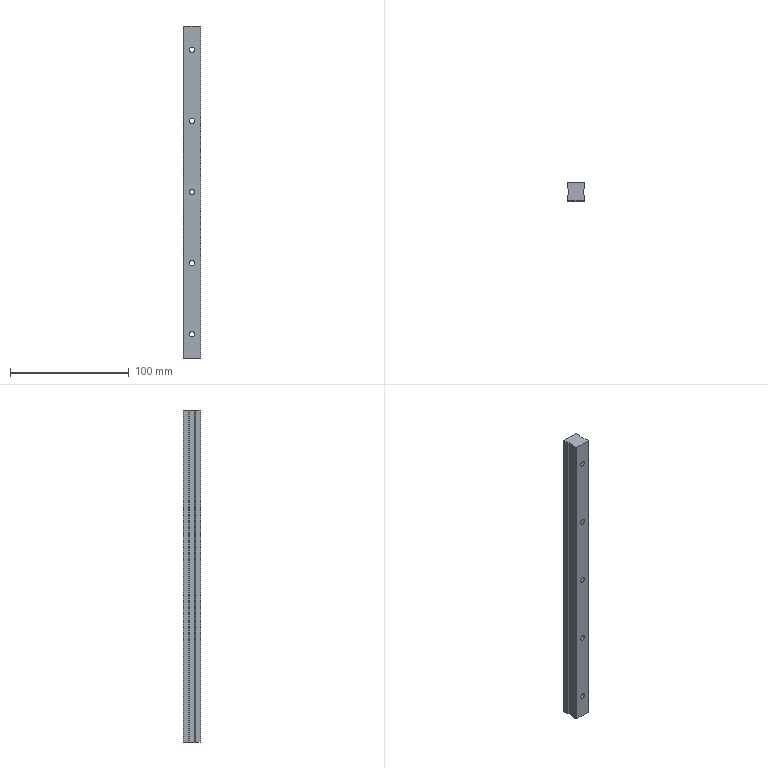Part | SolidWorks | features BaseBody 1 | 1 solid | 41 faces | box 15 x 15 x 280 mm | volume 57550 mm3 | plane 21 | cylinder 20 | commonest cylinder face diameters 4.5 x10 7.5 x10
STEP:
#1=CARTESIAN_POINT('',(0.,9.7,-117.75));
#2=VERTEX_POINT('',#1);
#3=CARTESIAN_POINT('',(0.,0.,-117.75));
#4=VERTEX_POINT('',#3);
#5=CARTESIAN_POINT('',(0.,15.,-117.75));
#6=DIRECTION('',(0.,-1.,0.));
#7=VECTOR('',#6,1000.);
#8=LINE('',#5,#7);
#9=EDGE_CURVE('',#2,#4,#8,.T.);
#10=ORIENTED_EDGE('',*,*,#9,.F.);
#11=CARTESIAN_POINT('',(0.,9.7,-122.25));
#12=VERTEX_POINT('',#11);
#13=CARTESIAN_POINT('',(0.,9.7,-120.));
#14=DIRECTION('',(0.,-1.,0.));
#15=DIRECTION('',(0.,0.,-1.));
#16=AXIS2_PLACEMENT_3D('',#13,#14,#15);
#17=CIRCLE('',#16,2.25);
#18=EDGE_CURVE('',#12,#2,#17,.T.);
#19=ORIENTED_EDGE('',*,*,#18,.F.);
#20=CARTESIAN_POINT('',(0.,0.,-122.25));
#21=VERTEX_POINT('',#20);
#22=CARTESIAN_POINT('',(0.,15.,-122.25));
#23=DIRECTION('',(0.,-1.,0.));
#24=VECTOR('',#23,1000.);
#25=LINE('',#22,#24);
#26=EDGE_CURVE('',#12,#21,#25,.T.);
#27=ORIENTED_EDGE('',*,*,#26,.T.);
#28=CARTESIAN_POINT('',(0.,0.,-120.));
#29=DIRECTION('',(0.,-1.,0.));
#30=DIRECTION('',(0.,0.,-1.));
#31=AXIS2_PLACEMENT_3D('',#28,#29,#30);
#32=CIRCLE('',#31,2.25);
#33=EDGE_CURVE('',#21,#4,#32,.T.);
#34=ORIENTED_EDGE('',*,*,#33,.T.);
#35=EDGE_LOOP('',(#10,#19,#27,#34));
#36=FACE_OUTER_BOUND('',#35,.T.);
#37=CARTESIAN_POINT('',(0.,15.,-120.));
#38=DIRECTION('',(0.,-1.,0.));
#39=DIRECTION('',(0.,0.,-1.));
#40=AXIS2_PLACEMENT_3D('',#37,#38,#39);
#41=CYLINDRICAL_SURFACE('',#40,2.25);
#42=ADVANCED_FACE('',(#36),#41,.F.);
#43=ORIENTED_EDGE('',*,*,#18,.T.);
#44=CARTESIAN_POINT('',(0.,9.7,-120.));
#45=DIRECTION('',(0.,-1.,0.));
#46=DIRECTION('',(0.,0.,-1.));
#47=AXIS2_PLACEMENT_3D('',#44,#45,#46);
#48=CIRCLE('',#47,2.25);
#49=EDGE_CURVE('',#2,#12,#48,.T.);
#50=ORIENTED_EDGE('',*,*,#49,.T.);
#51=EDGE_LOOP('',(#43,#50));
#52=FACE_BOUND('',#51,.T.);
#53=CARTESIAN_POINT('',(0.,9.7,-123.75));
#54=VERTEX_POINT('',#53);
#55=CARTESIAN_POINT('',(0.,9.7,-116.25));
#56=VERTEX_POINT('',#55);
#57=CARTESIAN_POINT('',(0.,9.7,-120.));
#58=DIRECTION('',(0.,-1.,0.));
#59=DIRECTION('',(0.,0.,-1.));
#60=AXIS2_PLACEMENT_3D('',#57,#58,#59);
#61=CIRCLE('',#60,3.75);
#62=EDGE_CURVE('',#54,#56,#61,.T.);
#63=ORIENTED_EDGE('',*,*,#62,.F.);
#64=CARTESIAN_POINT('',(0.,9.7,-120.));
#65=DIRECTION('',(0.,-1.,0.));
#66=DIRECTION('',(0.,0.,-1.));
#67=AXIS2_PLACEMENT_3D('',#64,#65,#66);
#68=CIRCLE('',#67,3.75);
#69=EDGE_CURVE('',#56,#54,#68,.T.);
#70=ORIENTED_EDGE('',*,*,#69,.F.);
#71=EDGE_LOOP('',(#63,#70));
#72=FACE_OUTER_BOUND('',#71,.T.);
#73=CARTESIAN_POINT('',(0.,9.7,-116.25));
#74=DIRECTION('',(0.,1.,0.));
#75=DIRECTION('',(1.,0.,0.));
#76=AXIS2_PLACEMENT_3D('',#73,#74,#75);
#77=PLANE('',#76);
#78=ADVANCED_FACE('',(#52,#72),#77,.T.);
#79=CARTESIAN_POINT('',(0.,15.,-116.25));
#80=VERTEX_POINT('',#79);
#81=CARTESIAN_POINT('',(0.,15.,-116.25));
#82=DIRECTION('',(0.,-1.,0.));
#83=VECTOR('',#82,1000.);
#84=LINE('',#81,#83);
#85=EDGE_CURVE('',#80,#56,#84,.T.);
#86=ORIENTED_EDGE('',*,*,#85,.F.);
#87=CARTESIAN_POINT('',(0.,15.,-123.75));
#88=VERTEX_POINT('',#87);
#89=CARTESIAN_POINT('',(0.,15.,-120.));
#90=DIRECTION('',(0.,-1.,0.));
#91=DIRECTION('',(0.,0.,-1.));
#92=AXIS2_PLACEMENT_3D('',#89,#90,#91);
#93=CIRCLE('',#92,3.75);
#94=EDGE_CURVE('',#88,#80,#93,.T.);
#95=ORIENTED_EDGE('',*,*,#94,.F.);
#96=CARTESIAN_POINT('',(0.,15.,-123.75));
#97=DIRECTION('',(0.,-1.,0.));
#98=VECTOR('',#97,1000.);
#99=LINE('',#96,#98);
#100=EDGE_CURVE('',#88,#54,#99,.T.);
#101=ORIENTED_EDGE('',*,*,#100,.T.);
#102=ORIENTED_EDGE('',*,*,#62,.T.);
#103=EDGE_LOOP('',(#86,#95,#101,#102));
#104=FACE_OUTER_BOUND('',#103,.T.);
#105=CARTESIAN_POINT('',(0.,15.,-120.));
#106=DIRECTION('',(0.,-1.,0.));
#107=DIRECTION('',(0.,0.,-1.));
#108=AXIS2_PLACEMENT_3D('',#105,#106,#107);
#109=CYLINDRICAL_SURFACE('',#108,3.75);
#110=ADVANCED_FACE('',(#104),#109,.F.);
#111=CARTESIAN_POINT('',(0.,9.7,-57.75));
#112=VERTEX_POINT('',#111);
#113=CARTESIAN_POINT('',(0.,0.,-57.75));
#114=VERTEX_POINT('',#113);
#115=CARTESIAN_POINT('',(0.,15.,-57.75));
#116=DIRECTION('',(0.,-1.,0.));
#117=VECTOR('',#116,1000.);
#118=LINE('',#115,#117);
#119=EDGE_CURVE('',#112,#114,#118,.T.);
#120=ORIENTED_EDGE('',*,*,#119,.F.);
#121=CARTESIAN_POINT('',(0.,9.7,-62.25));
#122=VERTEX_POINT('',#121);
#123=CARTESIAN_POINT('',(0.,9.7,-60.));
#124=DIRECTION('',(0.,-1.,0.));
#125=DIRECTION('',(0.,0.,-1.));
#126=AXIS2_PLACEMENT_3D('',#123,#124,#125);
#127=CIRCLE('',#126,2.25);
#128=EDGE_CURVE('',#122,#112,#127,.T.);
#129=ORIENTED_EDGE('',*,*,#128,.F.);
#130=CARTESIAN_POINT('',(0.,0.,-62.25));
#131=VERTEX_POINT('',#130);
#132=CARTESIAN_POINT('',(0.,15.,-62.25));
#133=DIRECTION('',(0.,-1.,0.));
#134=VECTOR('',#133,1000.);
#135=LINE('',#132,#134);
#136=EDGE_CURVE('',#122,#131,#135,.T.);
#137=ORIENTED_EDGE('',*,*,#136,.T.);
#138=CARTESIAN_POINT('',(0.,0.,-60.));
#139=DIRECTION('',(0.,-1.,0.));
#140=DIRECTION('',(0.,0.,-1.));
#141=AXIS2_PLACEMENT_3D('',#138,#139,#140);
#142=CIRCLE('',#141,2.25);
#143=EDGE_CURVE('',#131,#114,#142,.T.);
#144=ORIENTED_EDGE('',*,*,#143,.T.);
#145=EDGE_LOOP('',(#120,#129,#137,#144));
#146=FACE_OUTER_BOUND('',#145,.T.);
#147=CARTESIAN_POINT('',(0.,15.,-60.));
#148=DIRECTION('',(0.,-1.,0.));
#149=DIRECTION('',(0.,0.,-1.));
#150=AXIS2_PLACEMENT_3D('',#147,#148,#149);
#151=CYLINDRICAL_SURFACE('',#150,2.25);
#152=ADVANCED_FACE('',(#146),#151,.F.);
#153=ORIENTED_EDGE('',*,*,#128,.T.);
#154=CARTESIAN_POINT('',(0.,9.7,-60.));
#155=DIRECTION('',(0.,-1.,0.));
#156=DIRECTION('',(0.,0.,-1.));
#157=AXIS2_PLACEMENT_3D('',#154,#155,#156);
#158=CIRCLE('',#157,2.25);
#159=EDGE_CURVE('',#112,#122,#158,.T.);
#160=ORIENTED_EDGE('',*,*,#159,.T.);
#161=EDGE_LOOP('',(#153,#160));
#162=FACE_BOUND('',#161,.T.);
#163=CARTESIAN_POINT('',(0.,9.7,-63.75));
#164=VERTEX_POINT('',#163);
#165=CARTESIAN_POINT('',(0.,9.7,-56.25));
#166=VERTEX_POINT('',#165);
#167=CARTESIAN_POINT('',(0.,9.7,-60.));
#168=DIRECTION('',(0.,-1.,0.));
#169=DIRECTION('',(0.,0.,-1.));
#170=AXIS2_PLACEMENT_3D('',#167,#168,#169);
#171=CIRCLE('',#170,3.75);
#172=EDGE_CURVE('',#164,#166,#171,.T.);
#173=ORIENTED_EDGE('',*,*,#172,.F.);
#174=CARTESIAN_POINT('',(0.,9.7,-60.));
#175=DIRECTION('',(0.,-1.,0.));
#176=DIRECTION('',(0.,0.,-1.));
#177=AXIS2_PLACEMENT_3D('',#174,#175,#176);
#178=CIRCLE('',#177,3.75);
#179=EDGE_CURVE('',#166,#164,#178,.T.);
#180=ORIENTED_EDGE('',*,*,#179,.F.);
#181=EDGE_LOOP('',(#173,#180));
#182=FACE_OUTER_BOUND('',#181,.T.);
#183=CARTESIAN_POINT('',(0.,9.7,-56.25));
#184=DIRECTION('',(0.,1.,0.));
#185=DIRECTION('',(1.,0.,0.));
#186=AXIS2_PLACEMENT_3D('',#183,#184,#185);
#187=PLANE('',#186);
#188=ADVANCED_FACE('',(#162,#182),#187,.T.);
#189=CARTESIAN_POINT('',(0.,15.,-56.25));
#190=VERTEX_POINT('',#189);
#191=CARTESIAN_POINT('',(0.,15.,-56.25));
#192=DIRECTION('',(0.,-1.,0.));
#193=VECTOR('',#192,1000.);
#194=LINE('',#191,#193);
#195=EDGE_CURVE('',#190,#166,#194,.T.);
#196=ORIENTED_EDGE('',*,*,#195,.F.);
#197=CARTESIAN_POINT('',(0.,15.,-63.75));
#198=VERTEX_POINT('',#197);
#199=CARTESIAN_POINT('',(0.,15.,-60.));
#200=DIRECTION('',(0.,-1.,0.));
#201=DIRECTION('',(0.,0.,-1.));
#202=AXIS2_PLACEMENT_3D('',#199,#200,#201);
#203=CIRCLE('',#202,3.75);
#204=EDGE_CURVE('',#198,#190,#203,.T.);
#205=ORIENTED_EDGE('',*,*,#204,.F.);
#206=CARTESIAN_POINT('',(0.,15.,-63.75));
#207=DIRECTION('',(0.,-1.,0.));
#208=VECTOR('',#207,1000.);
#209=LINE('',#206,#208);
#210=EDGE_CURVE('',#198,#164,#209,.T.);
#211=ORIENTED_EDGE('',*,*,#210,.T.);
#212=ORIENTED_EDGE('',*,*,#172,.T.);
#213=EDGE_LOOP('',(#196,#205,#211,#212));
#214=FACE_OUTER_BOUND('',#213,.T.);
#215=CARTESIAN_POINT('',(0.,15.,-60.));
#216=DIRECTION('',(0.,-1.,0.));
#217=DIRECTION('',(0.,0.,-1.));
#218=AXIS2_PLACEMENT_3D('',#215,#216,#217);
#219=CYLINDRICAL_SURFACE('',#218,3.75);
#220=ADVANCED_FACE('',(#214),#219,.F.);
#221=CARTESIAN_POINT('',(0.,9.7,2.25));
#222=VERTEX_POINT('',#221);
#223=CARTESIAN_POINT('',(0.,0.,2.25));
#224=VERTEX_POINT('',#223);
#225=CARTESIAN_POINT('',(0.,15.,2.25));
#226=DIRECTION('',(0.,-1.,0.));
#227=VECTOR('',#226,1000.);
#228=LINE('',#225,#227);
#229=EDGE_CURVE('',#222,#224,#228,.T.);
#230=ORIENTED_EDGE('',*,*,#229,.F.);
#231=CARTESIAN_POINT('',(0.,9.7,-2.25));
#232=VERTEX_POINT('',#231);
#233=CARTESIAN_POINT('',(0.,9.7,0.));
#234=DIRECTION('',(0.,-1.,0.));
#235=DIRECTION('',(0.,0.,-1.));
#236=AXIS2_PLACEMENT_3D('',#233,#234,#235);
#237=CIRCLE('',#236,2.25);
#238=EDGE_CURVE('',#232,#222,#237,.T.);
#239=ORIENTED_EDGE('',*,*,#238,.F.);
#240=CARTESIAN_POINT('',(0.,0.,-2.25));
#241=VERTEX_POINT('',#240);
#242=CARTESIAN_POINT('',(0.,15.,-2.25));
#243=DIRECTION('',(0.,-1.,0.));
#244=VECTOR('',#243,1000.);
#245=LINE('',#242,#244);
#246=EDGE_CURVE('',#232,#241,#245,.T.);
#247=ORIENTED_EDGE('',*,*,#246,.T.);
#248=CARTESIAN_POINT('',(0.,0.,0.));
#249=DIRECTION('',(0.,-1.,0.));
#250=DIRECTION('',(0.,0.,-1.));
#251=AXIS2_PLACEMENT_3D('',#248,#249,#250);
#252=CIRCLE('',#251,2.25);
#253=EDGE_CURVE('',#241,#224,#252,.T.);
#254=ORIENTED_EDGE('',*,*,#253,.T.);
#255=EDGE_LOOP('',(#230,#239,#247,#254));
#256=FACE_OUTER_BOUND('',#255,.T.);
#257=CARTESIAN_POINT('',(0.,15.,0.));
#258=DIRECTION('',(0.,-1.,0.));
#259=DIRECTION('',(0.,0.,-1.));
#260=AXIS2_PLACEMENT_3D('',#257,#258,#259);
#261=CYLINDRICAL_SURFACE('',#260,2.25);
#262=ADVANCED_FACE('',(#256),#261,.F.);
#263=ORIENTED_EDGE('',*,*,#238,.T.);
#264=CARTESIAN_POINT('',(0.,9.7,0.));
#265=DIRECTION('',(0.,-1.,0.));
#266=DIRECTION('',(0.,0.,-1.));
#267=AXIS2_PLACEMENT_3D('',#264,#265,#266);
#268=CIRCLE('',#267,2.25);
#269=EDGE_CURVE('',#222,#232,#268,.T.);
#270=ORIENTED_EDGE('',*,*,#269,.T.);
#271=EDGE_LOOP('',(#263,#270));
#272=FACE_BOUND('',#271,.T.);
#273=CARTESIAN_POINT('',(0.,9.7,-3.75));
#274=VERTEX_POINT('',#273);
#275=CARTESIAN_POINT('',(0.,9.7,3.75));
#276=VERTEX_POINT('',#275);
#277=CARTESIAN_POINT('',(0.,9.7,0.));
#278=DIRECTION('',(0.,-1.,0.));
#279=DIRECTION('',(0.,0.,-1.));
#280=AXIS2_PLACEMENT_3D('',#277,#278,#279);
#281=CIRCLE('',#280,3.75);
#282=EDGE_CURVE('',#274,#276,#281,.T.);
#283=ORIENTED_EDGE('',*,*,#282,.F.);
#284=CARTESIAN_POINT('',(0.,9.7,0.));
#285=DIRECTION('',(0.,-1.,0.));
#286=DIRECTION('',(0.,0.,-1.));
#287=AXIS2_PLACEMENT_3D('',#284,#285,#286);
#288=CIRCLE('',#287,3.75);
#289=EDGE_CURVE('',#276,#274,#288,.T.);
#290=ORIENTED_EDGE('',*,*,#289,.F.);
#291=EDGE_LOOP('',(#283,#290));
#292=FACE_OUTER_BOUND('',#291,.T.);
#293=CARTESIAN_POINT('',(0.,9.7,3.75));
#294=DIRECTION('',(0.,1.,0.));
#295=DIRECTION('',(1.,0.,0.));
#296=AXIS2_PLACEMENT_3D('',#293,#294,#295);
#297=PLANE('',#296);
#298=ADVANCED_FACE('',(#272,#292),#297,.T.);
#299=CARTESIAN_POINT('',(0.,15.,3.75));
#300=VERTEX_POINT('',#299);
#301=CARTESIAN_POINT('',(0.,15.,3.75));
#302=DIRECTION('',(0.,-1.,0.));
#303=VECTOR('',#302,1000.);
#304=LINE('',#301,#303);
#305=EDGE_CURVE('',#300,#276,#304,.T.);
#306=ORIENTED_EDGE('',*,*,#305,.F.);
#307=CARTESIAN_POINT('',(0.,15.,-3.75));
#308=VERTEX_POINT('',#307);
#309=CARTESIAN_POINT('',(0.,15.,0.));
#310=DIRECTION('',(0.,-1.,0.));
#311=DIRECTION('',(0.,0.,-1.));
#312=AXIS2_PLACEMENT_3D('',#309,#310,#311);
#313=CIRCLE('',#312,3.75);
#314=EDGE_CURVE('',#308,#300,#313,.T.);
#315=ORIENTED_EDGE('',*,*,#314,.F.);
#316=CARTESIAN_POINT('',(0.,15.,-3.75));
#317=DIRECTION('',(0.,-1.,0.));
#318=VECTOR('',#317,1000.);
#319=LINE('',#316,#318);
#320=EDGE_CURVE('',#308,#274,#319,.T.);
#321=ORIENTED_EDGE('',*,*,#320,.T.);
#322=ORIENTED_EDGE('',*,*,#282,.T.);
#323=EDGE_LOOP('',(#306,#315,#321,#322));
#324=FACE_OUTER_BOUND('',#323,.T.);
#325=CARTESIAN_POINT('',(0.,15.,0.));
#326=DIRECTION('',(0.,-1.,0.));
#327=DIRECTION('',(0.,0.,-1.));
#328=AXIS2_PLACEMENT_3D('',#325,#326,#327);
#329=CYLINDRICAL_SURFACE('',#328,3.75);
#330=ADVANCED_FACE('',(#324),#329,.F.);
#331=CARTESIAN_POINT('',(0.,9.7,62.25));
#332=VERTEX_POINT('',#331);
#333=CARTESIAN_POINT('',(0.,0.,62.25));
#334=VERTEX_POINT('',#333);
#335=CARTESIAN_POINT('',(0.,15.,62.25));
#336=DIRECTION('',(0.,-1.,0.));
#337=VECTOR('',#336,1000.);
#338=LINE('',#335,#337);
#339=EDGE_CURVE('',#332,#334,#338,.T.);
#340=ORIENTED_EDGE('',*,*,#339,.F.);
#341=CARTESIAN_POINT('',(0.,9.7,57.75));
#342=VERTEX_POINT('',#341);
#343=CARTESIAN_POINT('',(0.,9.7,60.));
#344=DIRECTION('',(0.,-1.,0.));
#345=DIRECTION('',(0.,0.,-1.));
#346=AXIS2_PLACEMENT_3D('',#343,#344,#345);
#347=CIRCLE('',#346,2.25);
#348=EDGE_CURVE('',#342,#332,#347,.T.);
#349=ORIENTED_EDGE('',*,*,#348,.F.);
#350=CARTESIAN_POINT('',(0.,0.,57.75));
#351=VERTEX_POINT('',#350);
#352=CARTESIAN_POINT('',(0.,15.,57.75));
#353=DIRECTION('',(0.,-1.,0.));
#354=VECTOR('',#353,1000.);
#355=LINE('',#352,#354);
#356=EDGE_CURVE('',#342,#351,#355,.T.);
#357=ORIENTED_EDGE('',*,*,#356,.T.);
#358=CARTESIAN_POINT('',(0.,0.,60.));
#359=DIRECTION('',(0.,-1.,0.));
#360=DIRECTION('',(0.,0.,-1.));
#361=AXIS2_PLACEMENT_3D('',#358,#359,#360);
#362=CIRCLE('',#361,2.25);
#363=EDGE_CURVE('',#351,#334,#362,.T.);
#364=ORIENTED_EDGE('',*,*,#363,.T.);
#365=EDGE_LOOP('',(#340,#349,#357,#364));
#366=FACE_OUTER_BOUND('',#365,.T.);
#367=CARTESIAN_POINT('',(0.,15.,60.));
#368=DIRECTION('',(0.,-1.,0.));
#369=DIRECTION('',(0.,0.,-1.));
#370=AXIS2_PLACEMENT_3D('',#367,#368,#369);
#371=CYLINDRICAL_SURFACE('',#370,2.25);
#372=ADVANCED_FACE('',(#366),#371,.F.);
#373=ORIENTED_EDGE('',*,*,#348,.T.);
#374=CARTESIAN_POINT('',(0.,9.7,60.));
#375=DIRECTION('',(0.,-1.,0.));
#376=DIRECTION('',(0.,0.,-1.));
#377=AXIS2_PLACEMENT_3D('',#374,#375,#376);
#378=CIRCLE('',#377,2.25);
#379=EDGE_CURVE('',#332,#342,#378,.T.);
#380=ORIENTED_EDGE('',*,*,#379,.T.);
#381=EDGE_LOOP('',(#373,#380));
#382=FACE_BOUND('',#381,.T.);
#383=CARTESIAN_POINT('',(0.,9.7,56.25));
#384=VERTEX_POINT('',#383);
#385=CARTESIAN_POINT('',(0.,9.7,63.75));
#386=VERTEX_POINT('',#385);
#387=CARTESIAN_POINT('',(0.,9.7,60.));
#388=DIRECTION('',(0.,-1.,0.));
#389=DIRECTION('',(0.,0.,-1.));
#390=AXIS2_PLACEMENT_3D('',#387,#388,#389);
#391=CIRCLE('',#390,3.75);
#392=EDGE_CURVE('',#384,#386,#391,.T.);
#393=ORIENTED_EDGE('',*,*,#392,.F.);
#394=CARTESIAN_POINT('',(0.,9.7,60.));
#395=DIRECTION('',(0.,-1.,0.));
#396=DIRECTION('',(0.,0.,-1.));
#397=AXIS2_PLACEMENT_3D('',#394,#395,#396);
#398=CIRCLE('',#397,3.75);
#399=EDGE_CURVE('',#386,#384,#398,.T.);
#400=ORIENTED_EDGE('',*,*,#399,.F.);
#401=EDGE_LOOP('',(#393,#400));
#402=FACE_OUTER_BOUND('',#401,.T.);
#403=CARTESIAN_POINT('',(0.,9.7,63.75));
#404=DIRECTION('',(0.,1.,0.));
#405=DIRECTION('',(1.,0.,0.));
#406=AXIS2_PLACEMENT_3D('',#403,#404,#405);
#407=PLANE('',#406);
#408=ADVANCED_FACE('',(#382,#402),#407,.T.);
#409=CARTESIAN_POINT('',(0.,15.,63.75));
#410=VERTEX_POINT('',#409);
#411=CARTESIAN_POINT('',(0.,15.,63.75));
#412=DIRECTION('',(0.,-1.,0.));
#413=VECTOR('',#412,1000.);
#414=LINE('',#411,#413);
#415=EDGE_CURVE('',#410,#386,#414,.T.);
#416=ORIENTED_EDGE('',*,*,#415,.F.);
#417=CARTESIAN_POINT('',(0.,15.,56.25));
#418=VERTEX_POINT('',#417);
#419=CARTESIAN_POINT('',(0.,15.,60.));
#420=DIRECTION('',(0.,-1.,0.));
#421=DIRECTION('',(0.,0.,-1.));
#422=AXIS2_PLACEMENT_3D('',#419,#420,#421);
#423=CIRCLE('',#422,3.75);
#424=EDGE_CURVE('',#418,#410,#423,.T.);
#425=ORIENTED_EDGE('',*,*,#424,.F.);
#426=CARTESIAN_POINT('',(0.,15.,56.25));
#427=DIRECTION('',(0.,-1.,0.));
#428=VECTOR('',#427,1000.);
#429=LINE('',#426,#428);
#430=EDGE_CURVE('',#418,#384,#429,.T.);
#431=ORIENTED_EDGE('',*,*,#430,.T.);
#432=ORIENTED_EDGE('',*,*,#392,.T.);
#433=EDGE_LOOP('',(#416,#425,#431,#432));
#434=FACE_OUTER_BOUND('',#433,.T.);
#435=CARTESIAN_POINT('',(0.,15.,60.));
#436=DIRECTION('',(0.,-1.,0.));
#437=DIRECTION('',(0.,0.,-1.));
#438=AXIS2_PLACEMENT_3D('',#435,#436,#437);
#439=CYLINDRICAL_SURFACE('',#438,3.75);
#440=ADVANCED_FACE('',(#434),#439,.F.);
#441=CARTESIAN_POINT('',(0.,9.7,122.25));
#442=VERTEX_POINT('',#441);
#443=CARTESIAN_POINT('',(0.,0.,122.25));
#444=VERTEX_POINT('',#443);
#445=CARTESIAN_POINT('',(0.,15.,122.25));
#446=DIRECTION('',(0.,-1.,0.));
#447=VECTOR('',#446,1000.);
#448=LINE('',#445,#447);
#449=EDGE_CURVE('',#442,#444,#448,.T.);
#450=ORIENTED_EDGE('',*,*,#449,.F.);
#451=CARTESIAN_POINT('',(0.,9.7,117.75));
#452=VERTEX_POINT('',#451);
#453=CARTESIAN_POINT('',(0.,9.7,120.));
#454=DIRECTION('',(0.,-1.,0.));
#455=DIRECTION('',(0.,0.,-1.));
#456=AXIS2_PLACEMENT_3D('',#453,#454,#455);
#457=CIRCLE('',#456,2.25);
#458=EDGE_CURVE('',#452,#442,#457,.T.);
#459=ORIENTED_EDGE('',*,*,#458,.F.);
#460=CARTESIAN_POINT('',(0.,0.,117.75));
#461=VERTEX_POINT('',#460);
#462=CARTESIAN_POINT('',(0.,15.,117.75));
#463=DIRECTION('',(0.,-1.,0.));
#464=VECTOR('',#463,1000.);
#465=LINE('',#462,#464);
#466=EDGE_CURVE('',#452,#461,#465,.T.);
#467=ORIENTED_EDGE('',*,*,#466,.T.);
#468=CARTESIAN_POINT('',(0.,0.,120.));
#469=DIRECTION('',(0.,-1.,0.));
#470=DIRECTION('',(0.,0.,-1.));
#471=AXIS2_PLACEMENT_3D('',#468,#469,#470);
#472=CIRCLE('',#471,2.25);
#473=EDGE_CURVE('',#461,#444,#472,.T.);
#474=ORIENTED_EDGE('',*,*,#473,.T.);
#475=EDGE_LOOP('',(#450,#459,#467,#474));
#476=FACE_OUTER_BOUND('',#475,.T.);
#477=CARTESIAN_POINT('',(0.,15.,120.));
#478=DIRECTION('',(0.,-1.,0.));
#479=DIRECTION('',(0.,0.,-1.));
#480=AXIS2_PLACEMENT_3D('',#477,#478,#479);
#481=CYLINDRICAL_SURFACE('',#480,2.25);
#482=ADVANCED_FACE('',(#476),#481,.F.);
#483=ORIENTED_EDGE('',*,*,#458,.T.);
#484=CARTESIAN_POINT('',(0.,9.7,120.));
#485=DIRECTION('',(0.,-1.,0.));
#486=DIRECTION('',(0.,0.,-1.));
#487=AXIS2_PLACEMENT_3D('',#484,#485,#486);
#488=CIRCLE('',#487,2.25);
#489=EDGE_CURVE('',#442,#452,#488,.T.);
#490=ORIENTED_EDGE('',*,*,#489,.T.);
#491=EDGE_LOOP('',(#483,#490));
#492=FACE_BOUND('',#491,.T.);
#493=CARTESIAN_POINT('',(0.,9.7,116.25));
#494=VERTEX_POINT('',#493);
#495=CARTESIAN_POINT('',(0.,9.7,123.75));
#496=VERTEX_POINT('',#495);
#497=CARTESIAN_POINT('',(0.,9.7,120.));
#498=DIRECTION('',(0.,-1.,0.));
#499=DIRECTION('',(0.,0.,-1.));
#500=AXIS2_PLACEMENT_3D('',#497,#498,#499);
#501=CIRCLE('',#500,3.75);
#502=EDGE_CURVE('',#494,#496,#501,.T.);
#503=ORIENTED_EDGE('',*,*,#502,.F.);
#504=CARTESIAN_POINT('',(0.,9.7,120.));
#505=DIRECTION('',(0.,-1.,0.));
#506=DIRECTION('',(0.,0.,-1.));
#507=AXIS2_PLACEMENT_3D('',#504,#505,#506);
#508=CIRCLE('',#507,3.75);
#509=EDGE_CURVE('',#496,#494,#508,.T.);
#510=ORIENTED_EDGE('',*,*,#509,.F.);
#511=EDGE_LOOP('',(#503,#510));
#512=FACE_OUTER_BOUND('',#511,.T.);
#513=CARTESIAN_POINT('',(0.,9.7,123.75));
#514=DIRECTION('',(0.,1.,0.));
#515=DIRECTION('',(1.,0.,0.));
#516=AXIS2_PLACEMENT_3D('',#513,#514,#515);
#517=PLANE('',#516);
#518=ADVANCED_FACE('',(#492,#512),#517,.T.);
#519=CARTESIAN_POINT('',(0.,15.,123.75));
#520=VERTEX_POINT('',#519);
#521=CARTESIAN_POINT('',(0.,15.,123.75));
#522=DIRECTION('',(0.,-1.,0.));
#523=VECTOR('',#522,1000.);
#524=LINE('',#521,#523);
#525=EDGE_CURVE('',#520,#496,#524,.T.);
#526=ORIENTED_EDGE('',*,*,#525,.F.);
#527=CARTESIAN_POINT('',(0.,15.,116.25));
#528=VERTEX_POINT('',#527);
#529=CARTESIAN_POINT('',(0.,15.,120.));
#530=DIRECTION('',(0.,-1.,0.));
#531=DIRECTION('',(0.,0.,-1.));
#532=AXIS2_PLACEMENT_3D('',#529,#530,#531);
#533=CIRCLE('',#532,3.75);
#534=EDGE_CURVE('',#528,#520,#533,.T.);
#535=ORIENTED_EDGE('',*,*,#534,.F.);
#536=CARTESIAN_POINT('',(0.,15.,116.25));
#537=DIRECTION('',(0.,-1.,0.));
#538=VECTOR('',#537,1000.);
#539=LINE('',#536,#538);
#540=EDGE_CURVE('',#528,#494,#539,.T.);
#541=ORIENTED_EDGE('',*,*,#540,.T.);
#542=ORIENTED_EDGE('',*,*,#502,.T.);
#543=EDGE_LOOP('',(#526,#535,#541,#542));
#544=FACE_OUTER_BOUND('',#543,.T.);
#545=CARTESIAN_POINT('',(0.,15.,120.));
#546=DIRECTION('',(0.,-1.,0.));
#547=DIRECTION('',(0.,0.,-1.));
#548=AXIS2_PLACEMENT_3D('',#545,#546,#547);
#549=CYLINDRICAL_SURFACE('',#548,3.75);
#550=ADVANCED_FACE('',(#544),#549,.F.);
#551=CARTESIAN_POINT('',(-7.5,0.7,140.));
#552=VERTEX_POINT('',#551);
#553=CARTESIAN_POINT('',(-6.8,0.,140.));
#554=VERTEX_POINT('',#553);
#555=CARTESIAN_POINT('',(-6.8,0.,140.));
#556=DIRECTION('',(0.7071,-0.7071,0.));
#557=VECTOR('',#556,1000.);
#558=LINE('',#555,#557);
#559=EDGE_CURVE('',#552,#554,#558,.T.);
#560=ORIENTED_EDGE('',*,*,#559,.F.);
#561=CARTESIAN_POINT('',(-7.5,0.7,-140.));
#562=VERTEX_POINT('',#561);
#563=CARTESIAN_POINT('',(-7.5,0.7,140.));
#564=DIRECTION('',(0.,0.,1.));
#565=VECTOR('',#564,1000.);
#566=LINE('',#563,#565);
#567=EDGE_CURVE('',#562,#552,#566,.T.);
#568=ORIENTED_EDGE('',*,*,#567,.F.);
#569=CARTESIAN_POINT('',(-6.8,0.,-140.));
#570=VERTEX_POINT('',#569);
#571=CARTESIAN_POINT('',(-3.4,-3.4,-140.));
#572=DIRECTION('',(-0.7071,0.7071,0.));
#573=VECTOR('',#572,1000.);
#574=LINE('',#571,#573);
#575=EDGE_CURVE('',#570,#562,#574,.T.);
#576=ORIENTED_EDGE('',*,*,#575,.F.);
#577=CARTESIAN_POINT('',(-6.8,0.,140.));
#578=DIRECTION('',(0.,0.,-1.));
#579=VECTOR('',#578,1000.);
#580=LINE('',#577,#579);
#581=EDGE_CURVE('',#554,#570,#580,.T.);
#582=ORIENTED_EDGE('',*,*,#581,.F.);
#583=EDGE_LOOP('',(#560,#568,#576,#582));
#584=FACE_OUTER_BOUND('',#583,.T.);
#585=CARTESIAN_POINT('',(-6.8,0.,140.));
#586=DIRECTION('',(0.7071,0.7071,0.));
#587=DIRECTION('',(0.,0.,-1.));
#588=AXIS2_PLACEMENT_3D('',#585,#586,#587);
#589=PLANE('',#588);
#590=ADVANCED_FACE('',(#584),#589,.F.);
#591=CARTESIAN_POINT('',(6.8,0.,140.));
#592=VERTEX_POINT('',#591);
#593=CARTESIAN_POINT('',(7.5,0.7,140.));
#594=VERTEX_POINT('',#593);
#595=CARTESIAN_POINT('',(7.5,0.7,140.));
#596=DIRECTION('',(0.7071,0.7071,0.));
#597=VECTOR('',#596,1000.);
#598=LINE('',#595,#597);
#599=EDGE_CURVE('',#592,#594,#598,.T.);
#600=ORIENTED_EDGE('',*,*,#599,.F.);
#601=CARTESIAN_POINT('',(6.8,0.,-140.));
#602=VERTEX_POINT('',#601);
#603=CARTESIAN_POINT('',(6.8,0.,140.));
#604=DIRECTION('',(0.,0.,1.));
#605=VECTOR('',#604,1000.);
#606=LINE('',#603,#605);
#607=EDGE_CURVE('',#602,#592,#606,.T.);
#608=ORIENTED_EDGE('',*,*,#607,.F.);
#609=CARTESIAN_POINT('',(7.5,0.7,-140.));
#610=VERTEX_POINT('',#609);
#611=CARTESIAN_POINT('',(3.4,-3.4,-140.));
#612=DIRECTION('',(-0.7071,-0.7071,0.));
#613=VECTOR('',#612,1000.);
#614=LINE('',#611,#613);
#615=EDGE_CURVE('',#610,#602,#614,.T.);
#616=ORIENTED_EDGE('',*,*,#615,.F.);
#617=CARTESIAN_POINT('',(7.5,0.7,140.));
#618=DIRECTION('',(0.,0.,-1.));
#619=VECTOR('',#618,1000.);
#620=LINE('',#617,#619);
#621=EDGE_CURVE('',#594,#610,#620,.T.);
#622=ORIENTED_EDGE('',*,*,#621,.F.);
#623=EDGE_LOOP('',(#600,#608,#616,#622));
#624=FACE_OUTER_BOUND('',#623,.T.);
#625=CARTESIAN_POINT('',(7.5,0.7,140.));
#626=DIRECTION('',(-0.7071,0.7071,0.));
#627=DIRECTION('',(0.,0.,1.));
#628=AXIS2_PLACEMENT_3D('',#625,#626,#627);
#629=PLANE('',#628);
#630=ADVANCED_FACE('',(#624),#629,.F.);
#631=CARTESIAN_POINT('',(7.5,4.3,-140.));
#632=VERTEX_POINT('',#631);
#633=CARTESIAN_POINT('',(7.5,0.,-140.));
#634=DIRECTION('',(0.,1.,0.));
#635=VECTOR('',#634,1000.);
#636=LINE('',#633,#635);
#637=EDGE_CURVE('',#610,#632,#636,.T.);
#638=ORIENTED_EDGE('',*,*,#637,.F.);
#639=ORIENTED_EDGE('',*,*,#615,.T.);
#640=CARTESIAN_POINT('',(-7.5,0.,-140.));
#641=DIRECTION('',(1.,0.,0.));
#642=VECTOR('',#641,1000.);
#643=LINE('',#640,#642);
#644=EDGE_CURVE('',#570,#602,#643,.T.);
#645=ORIENTED_EDGE('',*,*,#644,.F.);
#646=ORIENTED_EDGE('',*,*,#575,.T.);
#647=CARTESIAN_POINT('',(-7.5,4.3,-140.));
#648=VERTEX_POINT('',#647);
#649=CARTESIAN_POINT('',(-7.5,0.,-140.));
#650=DIRECTION('',(0.,-1.,0.));
#651=VECTOR('',#650,1000.);
#652=LINE('',#649,#651);
#653=EDGE_CURVE('',#648,#562,#652,.T.);
#654=ORIENTED_EDGE('',*,*,#653,.F.);
#655=CARTESIAN_POINT('',(-6.375,5.425,-140.));
#656=VERTEX_POINT('',#655);
#657=CARTESIAN_POINT('',(-7.5,4.3,-140.));
#658=DIRECTION('',(-0.7071,-0.7071,0.));
#659=VECTOR('',#658,1000.);
#660=LINE('',#657,#659);
#661=EDGE_CURVE('',#656,#648,#660,.T.);
#662=ORIENTED_EDGE('',*,*,#661,.F.);
#663=CARTESIAN_POINT('',(-6.375,9.65,-140.));
#664=VERTEX_POINT('',#663);
#665=CARTESIAN_POINT('',(-6.375,5.425,-140.));
#666=DIRECTION('',(0.,-1.,0.));
#667=VECTOR('',#666,1000.);
#668=LINE('',#665,#667);
#669=EDGE_CURVE('',#664,#656,#668,.T.);
#670=ORIENTED_EDGE('',*,*,#669,.F.);
#671=CARTESIAN_POINT('',(-7.5,10.775,-140.));
#672=VERTEX_POINT('',#671);
#673=CARTESIAN_POINT('',(-6.375,9.65,-140.));
#674=DIRECTION('',(0.7071,-0.7071,0.));
#675=VECTOR('',#674,1000.);
#676=LINE('',#673,#675);
#677=EDGE_CURVE('',#672,#664,#676,.T.);
#678=ORIENTED_EDGE('',*,*,#677,.F.);
#679=CARTESIAN_POINT('',(-7.5,15.,-140.));
#680=VERTEX_POINT('',#679);
#681=CARTESIAN_POINT('',(-7.5,10.775,-140.));
#682=DIRECTION('',(0.,-1.,0.));
#683=VECTOR('',#682,1000.);
#684=LINE('',#681,#683);
#685=EDGE_CURVE('',#680,#672,#684,.T.);
#686=ORIENTED_EDGE('',*,*,#685,.F.);
#687=CARTESIAN_POINT('',(7.5,15.,-140.));
#688=VERTEX_POINT('',#687);
#689=CARTESIAN_POINT('',(-7.5,15.,-140.));
#690=DIRECTION('',(-1.,0.,0.));
#691=VECTOR('',#690,1000.);
#692=LINE('',#689,#691);
#693=EDGE_CURVE('',#688,#680,#692,.T.);
#694=ORIENTED_EDGE('',*,*,#693,.F.);
#695=CARTESIAN_POINT('',(7.5,10.775,-140.));
#696=VERTEX_POINT('',#695);
#697=CARTESIAN_POINT('',(7.5,10.775,-140.));
#698=DIRECTION('',(0.,1.,0.));
#699=VECTOR('',#698,1000.);
#700=LINE('',#697,#699);
#701=EDGE_CURVE('',#696,#688,#700,.T.);
#702=ORIENTED_EDGE('',*,*,#701,.F.);
#703=CARTESIAN_POINT('',(6.375,9.65,-140.));
#704=VERTEX_POINT('',#703);
#705=CARTESIAN_POINT('',(6.375,9.65,-140.));
#706=DIRECTION('',(0.7071,0.7071,0.));
#707=VECTOR('',#706,1000.);
#708=LINE('',#705,#707);
#709=EDGE_CURVE('',#704,#696,#708,.T.);
#710=ORIENTED_EDGE('',*,*,#709,.F.);
#711=CARTESIAN_POINT('',(6.375,5.425,-140.));
#712=VERTEX_POINT('',#711);
#713=CARTESIAN_POINT('',(6.375,5.425,-140.));
#714=DIRECTION('',(0.,1.,0.));
#715=VECTOR('',#714,1000.);
#716=LINE('',#713,#715);
#717=EDGE_CURVE('',#712,#704,#716,.T.);
#718=ORIENTED_EDGE('',*,*,#717,.F.);
#719=CARTESIAN_POINT('',(7.5,4.3,-140.));
#720=DIRECTION('',(-0.7071,0.7071,0.));
#721=VECTOR('',#720,1000.);
#722=LINE('',#719,#721);
#723=EDGE_CURVE('',#632,#712,#722,.T.);
#724=ORIENTED_EDGE('',*,*,#723,.F.);
#725=EDGE_LOOP('',(#638,#639,#645,#646,#654,#662,#670,#678,#686,#694,#702,#710,#718,#724));
#726=FACE_OUTER_BOUND('',#725,.T.);
#727=CARTESIAN_POINT('',(0.,0.,-140.));
#728=DIRECTION('',(0.,0.,-1.));
#729=DIRECTION('',(0.,-1.,0.));
#730=AXIS2_PLACEMENT_3D('',#727,#728,#729);
#731=PLANE('',#730);
#732=ADVANCED_FACE('',(#726),#731,.T.);
#733=CARTESIAN_POINT('',(-7.5,0.,140.));
#734=DIRECTION('',(1.,0.,0.));
#735=VECTOR('',#734,1000.);
#736=LINE('',#733,#735);
#737=EDGE_CURVE('',#554,#592,#736,.T.);
#738=ORIENTED_EDGE('',*,*,#737,.T.);
#739=ORIENTED_EDGE('',*,*,#599,.T.);
#740=CARTESIAN_POINT('',(7.5,4.3,140.));
#741=VERTEX_POINT('',#740);
#742=CARTESIAN_POINT('',(7.5,0.,140.));
#743=DIRECTION('',(0.,1.,0.));
#744=VECTOR('',#743,1000.);
#745=LINE('',#742,#744);
#746=EDGE_CURVE('',#594,#741,#745,.T.);
#747=ORIENTED_EDGE('',*,*,#746,.T.);
#748=CARTESIAN_POINT('',(6.375,5.425,140.));
#749=VERTEX_POINT('',#748);
#750=CARTESIAN_POINT('',(7.5,4.3,140.));
#751=DIRECTION('',(-0.7071,0.7071,0.));
#752=VECTOR('',#751,1000.);
#753=LINE('',#750,#752);
#754=EDGE_CURVE('',#741,#749,#753,.T.);
#755=ORIENTED_EDGE('',*,*,#754,.T.);
#756=CARTESIAN_POINT('',(6.375,9.65,140.));
#757=VERTEX_POINT('',#756);
#758=CARTESIAN_POINT('',(6.375,5.425,140.));
#759=DIRECTION('',(0.,1.,0.));
#760=VECTOR('',#759,1000.);
#761=LINE('',#758,#760);
#762=EDGE_CURVE('',#749,#757,#761,.T.);
#763=ORIENTED_EDGE('',*,*,#762,.T.);
#764=CARTESIAN_POINT('',(7.5,10.775,140.));
#765=VERTEX_POINT('',#764);
#766=CARTESIAN_POINT('',(6.375,9.65,140.));
#767=DIRECTION('',(0.7071,0.7071,0.));
#768=VECTOR('',#767,1000.);
#769=LINE('',#766,#768);
#770=EDGE_CURVE('',#757,#765,#769,.T.);
#771=ORIENTED_EDGE('',*,*,#770,.T.);
#772=CARTESIAN_POINT('',(7.5,15.,140.));
#773=VERTEX_POINT('',#772);
#774=CARTESIAN_POINT('',(7.5,10.775,140.));
#775=DIRECTION('',(0.,1.,0.));
#776=VECTOR('',#775,1000.);
#777=LINE('',#774,#776);
#778=EDGE_CURVE('',#765,#773,#777,.T.);
#779=ORIENTED_EDGE('',*,*,#778,.T.);
#780=CARTESIAN_POINT('',(-7.5,15.,140.));
#781=VERTEX_POINT('',#780);
#782=CARTESIAN_POINT('',(-7.5,15.,140.));
#783=DIRECTION('',(-1.,0.,0.));
#784=VECTOR('',#783,1000.);
#785=LINE('',#782,#784);
#786=EDGE_CURVE('',#773,#781,#785,.T.);
#787=ORIENTED_EDGE('',*,*,#786,.T.);
#788=CARTESIAN_POINT('',(-7.5,10.775,140.));
#789=VERTEX_POINT('',#788);
#790=CARTESIAN_POINT('',(-7.5,10.775,140.));
#791=DIRECTION('',(0.,-1.,0.));
#792=VECTOR('',#791,1000.);
#793=LINE('',#790,#792);
#794=EDGE_CURVE('',#781,#789,#793,.T.);
#795=ORIENTED_EDGE('',*,*,#794,.T.);
#796=CARTESIAN_POINT('',(-6.375,9.65,140.));
#797=VERTEX_POINT('',#796);
#798=CARTESIAN_POINT('',(-6.375,9.65,140.));
#799=DIRECTION('',(0.7071,-0.7071,0.));
#800=VECTOR('',#799,1000.);
#801=LINE('',#798,#800);
#802=EDGE_CURVE('',#789,#797,#801,.T.);
#803=ORIENTED_EDGE('',*,*,#802,.T.);
#804=CARTESIAN_POINT('',(-6.375,5.425,140.));
#805=VERTEX_POINT('',#804);
#806=CARTESIAN_POINT('',(-6.375,5.425,140.));
#807=DIRECTION('',(0.,-1.,0.));
#808=VECTOR('',#807,1000.);
#809=LINE('',#806,#808);
#810=EDGE_CURVE('',#797,#805,#809,.T.);
#811=ORIENTED_EDGE('',*,*,#810,.T.);
#812=CARTESIAN_POINT('',(-7.5,4.3,140.));
#813=VERTEX_POINT('',#812);
#814=CARTESIAN_POINT('',(-7.5,4.3,140.));
#815=DIRECTION('',(-0.7071,-0.7071,0.));
#816=VECTOR('',#815,1000.);
#817=LINE('',#814,#816);
#818=EDGE_CURVE('',#805,#813,#817,.T.);
#819=ORIENTED_EDGE('',*,*,#818,.T.);
#820=CARTESIAN_POINT('',(-7.5,0.,140.));
#821=DIRECTION('',(0.,-1.,0.));
#822=VECTOR('',#821,1000.);
#823=LINE('',#820,#822);
#824=EDGE_CURVE('',#813,#552,#823,.T.);
#825=ORIENTED_EDGE('',*,*,#824,.T.);
#826=ORIENTED_EDGE('',*,*,#559,.T.);
#827=EDGE_LOOP('',(#738,#739,#747,#755,#763,#771,#779,#787,#795,#803,#811,#819,#825,#826));
#828=FACE_OUTER_BOUND('',#827,.T.);
#829=CARTESIAN_POINT('',(0.,0.,140.));
#830=DIRECTION('',(0.,0.,-1.));
#831=DIRECTION('',(0.,-1.,0.));
#832=AXIS2_PLACEMENT_3D('',#829,#830,#831);
#833=PLANE('',#832);
#834=ADVANCED_FACE('',(#828),#833,.F.);
#835=ORIENTED_EDGE('',*,*,#661,.T.);
#836=CARTESIAN_POINT('',(-7.5,4.3,140.));
#837=DIRECTION('',(0.,0.,-1.));
#838=VECTOR('',#837,1000.);
#839=LINE('',#836,#838);
#840=EDGE_CURVE('',#813,#648,#839,.T.);
#841=ORIENTED_EDGE('',*,*,#840,.F.);
#842=ORIENTED_EDGE('',*,*,#818,.F.);
#843=CARTESIAN_POINT('',(-6.375,5.425,140.));
#844=DIRECTION('',(0.,0.,-1.));
#845=VECTOR('',#844,1000.);
#846=LINE('',#843,#845);
#847=EDGE_CURVE('',#805,#656,#846,.T.);
#848=ORIENTED_EDGE('',*,*,#847,.T.);
#849=EDGE_LOOP('',(#835,#841,#842,#848));
#850=FACE_OUTER_BOUND('',#849,.T.);
#851=CARTESIAN_POINT('',(-7.5,4.3,140.));
#852=DIRECTION('',(0.7071,-0.7071,0.));
#853=DIRECTION('',(0.,0.,-1.));
#854=AXIS2_PLACEMENT_3D('',#851,#852,#853);
#855=PLANE('',#854);
#856=ADVANCED_FACE('',(#850),#855,.F.);
#857=ORIENTED_EDGE('',*,*,#669,.T.);
#858=ORIENTED_EDGE('',*,*,#847,.F.);
#859=ORIENTED_EDGE('',*,*,#810,.F.);
#860=CARTESIAN_POINT('',(-6.375,9.65,140.));
#861=DIRECTION('',(0.,0.,-1.));
#862=VECTOR('',#861,1000.);
#863=LINE('',#860,#862);
#864=EDGE_CURVE('',#797,#664,#863,.T.);
#865=ORIENTED_EDGE('',*,*,#864,.T.);
#866=EDGE_LOOP('',(#857,#858,#859,#865));
#867=FACE_OUTER_BOUND('',#866,.T.);
#868=CARTESIAN_POINT('',(-6.375,5.425,140.));
#869=DIRECTION('',(1.,0.,0.));
#870=DIRECTION('',(0.,1.,0.));
#871=AXIS2_PLACEMENT_3D('',#868,#869,#870);
#872=PLANE('',#871);
#873=ADVANCED_FACE('',(#867),#872,.F.);
#874=ORIENTED_EDGE('',*,*,#677,.T.);
#875=ORIENTED_EDGE('',*,*,#864,.F.);
#876=ORIENTED_EDGE('',*,*,#802,.F.);
#877=CARTESIAN_POINT('',(-7.5,10.775,140.));
#878=DIRECTION('',(0.,0.,-1.));
#879=VECTOR('',#878,1000.);
#880=LINE('',#877,#879);
#881=EDGE_CURVE('',#789,#672,#880,.T.);
#882=ORIENTED_EDGE('',*,*,#881,.T.);
#883=EDGE_LOOP('',(#874,#875,#876,#882));
#884=FACE_OUTER_BOUND('',#883,.T.);
#885=CARTESIAN_POINT('',(-6.375,9.65,140.));
#886=DIRECTION('',(0.7071,0.7071,0.));
#887=DIRECTION('',(0.,0.,-1.));
#888=AXIS2_PLACEMENT_3D('',#885,#886,#887);
#889=PLANE('',#888);
#890=ADVANCED_FACE('',(#884),#889,.F.);
#891=ORIENTED_EDGE('',*,*,#685,.T.);
#892=ORIENTED_EDGE('',*,*,#881,.F.);
#893=ORIENTED_EDGE('',*,*,#794,.F.);
#894=CARTESIAN_POINT('',(-7.5,15.,140.));
#895=DIRECTION('',(0.,0.,-1.));
#896=VECTOR('',#895,1000.);
#897=LINE('',#894,#896);
#898=EDGE_CURVE('',#781,#680,#897,.T.);
#899=ORIENTED_EDGE('',*,*,#898,.T.);
#900=EDGE_LOOP('',(#891,#892,#893,#899));
#901=FACE_OUTER_BOUND('',#900,.T.);
#902=CARTESIAN_POINT('',(-7.5,10.775,140.));
#903=DIRECTION('',(1.,0.,0.));
#904=DIRECTION('',(0.,1.,0.));
#905=AXIS2_PLACEMENT_3D('',#902,#903,#904);
#906=PLANE('',#905);
#907=ADVANCED_FACE('',(#901),#906,.F.);
#908=ORIENTED_EDGE('',*,*,#534,.T.);
#909=CARTESIAN_POINT('',(0.,15.,120.));
#910=DIRECTION('',(0.,-1.,0.));
#911=DIRECTION('',(0.,0.,-1.));
#912=AXIS2_PLACEMENT_3D('',#909,#910,#911);
#913=CIRCLE('',#912,3.75);
#914=EDGE_CURVE('',#520,#528,#913,.T.);
#915=ORIENTED_EDGE('',*,*,#914,.T.);
#916=EDGE_LOOP('',(#908,#915));
#917=FACE_BOUND('',#916,.T.);
#918=ORIENTED_EDGE('',*,*,#424,.T.);
#919=CARTESIAN_POINT('',(0.,15.,60.));
#920=DIRECTION('',(0.,-1.,0.));
#921=DIRECTION('',(0.,0.,-1.));
#922=AXIS2_PLACEMENT_3D('',#919,#920,#921);
#923=CIRCLE('',#922,3.75);
#924=EDGE_CURVE('',#410,#418,#923,.T.);
#925=ORIENTED_EDGE('',*,*,#924,.T.);
#926=EDGE_LOOP('',(#918,#925));
#927=FACE_BOUND('',#926,.T.);
#928=ORIENTED_EDGE('',*,*,#314,.T.);
#929=CARTESIAN_POINT('',(0.,15.,0.));
#930=DIRECTION('',(0.,-1.,0.));
#931=DIRECTION('',(0.,0.,-1.));
#932=AXIS2_PLACEMENT_3D('',#929,#930,#931);
#933=CIRCLE('',#932,3.75);
#934=EDGE_CURVE('',#300,#308,#933,.T.);
#935=ORIENTED_EDGE('',*,*,#934,.T.);
#936=EDGE_LOOP('',(#928,#935));
#937=FACE_BOUND('',#936,.T.);
#938=ORIENTED_EDGE('',*,*,#204,.T.);
#939=CARTESIAN_POINT('',(0.,15.,-60.));
#940=DIRECTION('',(0.,-1.,0.));
#941=DIRECTION('',(0.,0.,-1.));
#942=AXIS2_PLACEMENT_3D('',#939,#940,#941);
#943=CIRCLE('',#942,3.75);
#944=EDGE_CURVE('',#190,#198,#943,.T.);
#945=ORIENTED_EDGE('',*,*,#944,.T.);
#946=EDGE_LOOP('',(#938,#945));
#947=FACE_BOUND('',#946,.T.);
#948=ORIENTED_EDGE('',*,*,#94,.T.);
#949=CARTESIAN_POINT('',(0.,15.,-120.));
#950=DIRECTION('',(0.,-1.,0.));
#951=DIRECTION('',(0.,0.,-1.));
#952=AXIS2_PLACEMENT_3D('',#949,#950,#951);
#953=CIRCLE('',#952,3.75);
#954=EDGE_CURVE('',#80,#88,#953,.T.);
#955=ORIENTED_EDGE('',*,*,#954,.T.);
#956=EDGE_LOOP('',(#948,#955));
#957=FACE_BOUND('',#956,.T.);
#958=ORIENTED_EDGE('',*,*,#693,.T.);
#959=ORIENTED_EDGE('',*,*,#898,.F.);
#960=ORIENTED_EDGE('',*,*,#786,.F.);
#961=CARTESIAN_POINT('',(7.5,15.,140.));
#962=DIRECTION('',(0.,0.,-1.));
#963=VECTOR('',#962,1000.);
#964=LINE('',#961,#963);
#965=EDGE_CURVE('',#773,#688,#964,.T.);
#966=ORIENTED_EDGE('',*,*,#965,.T.);
#967=EDGE_LOOP('',(#958,#959,#960,#966));
#968=FACE_OUTER_BOUND('',#967,.T.);
#969=CARTESIAN_POINT('',(-7.5,15.,140.));
#970=DIRECTION('',(0.,-1.,0.));
#971=DIRECTION('',(0.,0.,-1.));
#972=AXIS2_PLACEMENT_3D('',#969,#970,#971);
#973=PLANE('',#972);
#974=ADVANCED_FACE('',(#917,#927,#937,#947,#957,#968),#973,.F.);
#975=ORIENTED_EDGE('',*,*,#701,.T.);
#976=ORIENTED_EDGE('',*,*,#965,.F.);
#977=ORIENTED_EDGE('',*,*,#778,.F.);
#978=CARTESIAN_POINT('',(7.5,10.775,140.));
#979=DIRECTION('',(0.,0.,-1.));
#980=VECTOR('',#979,1000.);
#981=LINE('',#978,#980);
#982=EDGE_CURVE('',#765,#696,#981,.T.);
#983=ORIENTED_EDGE('',*,*,#982,.T.);
#984=EDGE_LOOP('',(#975,#976,#977,#983));
#985=FACE_OUTER_BOUND('',#984,.T.);
#986=CARTESIAN_POINT('',(7.5,10.775,140.));
#987=DIRECTION('',(-1.,0.,0.));
#988=DIRECTION('',(0.,0.,1.));
#989=AXIS2_PLACEMENT_3D('',#986,#987,#988);
#990=PLANE('',#989);
#991=ADVANCED_FACE('',(#985),#990,.F.);
#992=ORIENTED_EDGE('',*,*,#709,.T.);
#993=ORIENTED_EDGE('',*,*,#982,.F.);
#994=ORIENTED_EDGE('',*,*,#770,.F.);
#995=CARTESIAN_POINT('',(6.375,9.65,140.));
#996=DIRECTION('',(0.,0.,-1.));
#997=VECTOR('',#996,1000.);
#998=LINE('',#995,#997);
#999=EDGE_CURVE('',#757,#704,#998,.T.);
#1000=ORIENTED_EDGE('',*,*,#999,.T.);
#1001=EDGE_LOOP('',(#992,#993,#994,#1000));
#1002=FACE_OUTER_BOUND('',#1001,.T.);
#1003=CARTESIAN_POINT('',(6.375,9.65,140.));
#1004=DIRECTION('',(-0.7071,0.7071,0.));
#1005=DIRECTION('',(0.,0.,1.));
#1006=AXIS2_PLACEMENT_3D('',#1003,#1004,#1005);
#1007=PLANE('',#1006);
#1008=ADVANCED_FACE('',(#1002),#1007,.F.);
#1009=ORIENTED_EDGE('',*,*,#717,.T.);
#1010=ORIENTED_EDGE('',*,*,#999,.F.);
#1011=ORIENTED_EDGE('',*,*,#762,.F.);
#1012=CARTESIAN_POINT('',(6.375,5.425,140.));
#1013=DIRECTION('',(0.,0.,-1.));
#1014=VECTOR('',#1013,1000.);
#1015=LINE('',#1012,#1014);
#1016=EDGE_CURVE('',#749,#712,#1015,.T.);
#1017=ORIENTED_EDGE('',*,*,#1016,.T.);
#1018=EDGE_LOOP('',(#1009,#1010,#1011,#1017));
#1019=FACE_OUTER_BOUND('',#1018,.T.);
#1020=CARTESIAN_POINT('',(6.375,5.425,140.));
#1021=DIRECTION('',(-1.,0.,0.));
#1022=DIRECTION('',(0.,0.,1.));
#1023=AXIS2_PLACEMENT_3D('',#1020,#1021,#1022);
#1024=PLANE('',#1023);
#1025=ADVANCED_FACE('',(#1019),#1024,.F.);
#1026=ORIENTED_EDGE('',*,*,#723,.T.);
#1027=ORIENTED_EDGE('',*,*,#1016,.F.);
#1028=ORIENTED_EDGE('',*,*,#754,.F.);
#1029=CARTESIAN_POINT('',(7.5,4.3,140.));
#1030=DIRECTION('',(0.,0.,-1.));
#1031=VECTOR('',#1030,1000.);
#1032=LINE('',#1029,#1031);
#1033=EDGE_CURVE('',#741,#632,#1032,.T.);
#1034=ORIENTED_EDGE('',*,*,#1033,.T.);
#1035=EDGE_LOOP('',(#1026,#1027,#1028,#1034));
#1036=FACE_OUTER_BOUND('',#1035,.T.);
#1037=CARTESIAN_POINT('',(7.5,4.3,140.));
#1038=DIRECTION('',(-0.7071,-0.7071,0.));
#1039=DIRECTION('',(-0.7071,0.7071,0.));
#1040=AXIS2_PLACEMENT_3D('',#1037,#1038,#1039);
#1041=PLANE('',#1040);
#1042=ADVANCED_FACE('',(#1036),#1041,.F.);
#1043=ORIENTED_EDGE('',*,*,#746,.F.);
#1044=ORIENTED_EDGE('',*,*,#621,.T.);
#1045=ORIENTED_EDGE('',*,*,#637,.T.);
#1046=ORIENTED_EDGE('',*,*,#1033,.F.);
#1047=EDGE_LOOP('',(#1043,#1044,#1045,#1046));
#1048=FACE_OUTER_BOUND('',#1047,.T.);
#1049=CARTESIAN_POINT('',(7.5,0.,140.));
#1050=DIRECTION('',(-1.,0.,0.));
#1051=DIRECTION('',(0.,0.,1.));
#1052=AXIS2_PLACEMENT_3D('',#1049,#1050,#1051);
#1053=PLANE('',#1052);
#1054=ADVANCED_FACE('',(#1048),#1053,.F.);
#1055=ORIENTED_EDGE('',*,*,#473,.F.);
#1056=CARTESIAN_POINT('',(0.,0.,120.));
#1057=DIRECTION('',(0.,-1.,0.));
#1058=DIRECTION('',(0.,0.,-1.));
#1059=AXIS2_PLACEMENT_3D('',#1056,#1057,#1058);
#1060=CIRCLE('',#1059,2.25);
#1061=EDGE_CURVE('',#444,#461,#1060,.T.);
#1062=ORIENTED_EDGE('',*,*,#1061,.F.);
#1063=EDGE_LOOP('',(#1055,#1062));
#1064=FACE_BOUND('',#1063,.T.);
#1065=ORIENTED_EDGE('',*,*,#363,.F.);
#1066=CARTESIAN_POINT('',(0.,0.,60.));
#1067=DIRECTION('',(0.,-1.,0.));
#1068=DIRECTION('',(0.,0.,-1.));
#1069=AXIS2_PLACEMENT_3D('',#1066,#1067,#1068);
#1070=CIRCLE('',#1069,2.25);
#1071=EDGE_CURVE('',#334,#351,#1070,.T.);
#1072=ORIENTED_EDGE('',*,*,#1071,.F.);
#1073=EDGE_LOOP('',(#1065,#1072));
#1074=FACE_BOUND('',#1073,.T.);
#1075=ORIENTED_EDGE('',*,*,#253,.F.);
#1076=CARTESIAN_POINT('',(0.,0.,0.));
#1077=DIRECTION('',(0.,-1.,0.));
#1078=DIRECTION('',(0.,0.,-1.));
#1079=AXIS2_PLACEMENT_3D('',#1076,#1077,#1078);
#1080=CIRCLE('',#1079,2.25);
#1081=EDGE_CURVE('',#224,#241,#1080,.T.);
#1082=ORIENTED_EDGE('',*,*,#1081,.F.);
#1083=EDGE_LOOP('',(#1075,#1082));
#1084=FACE_BOUND('',#1083,.T.);
#1085=ORIENTED_EDGE('',*,*,#143,.F.);
#1086=CARTESIAN_POINT('',(0.,0.,-60.));
#1087=DIRECTION('',(0.,-1.,0.));
#1088=DIRECTION('',(0.,0.,-1.));
#1089=AXIS2_PLACEMENT_3D('',#1086,#1087,#1088);
#1090=CIRCLE('',#1089,2.25);
#1091=EDGE_CURVE('',#114,#131,#1090,.T.);
#1092=ORIENTED_EDGE('',*,*,#1091,.F.);
#1093=EDGE_LOOP('',(#1085,#1092));
#1094=FACE_BOUND('',#1093,.T.);
#1095=ORIENTED_EDGE('',*,*,#33,.F.);
#1096=CARTESIAN_POINT('',(0.,0.,-120.));
#1097=DIRECTION('',(0.,-1.,0.));
#1098=DIRECTION('',(0.,0.,-1.));
#1099=AXIS2_PLACEMENT_3D('',#1096,#1097,#1098);
#1100=CIRCLE('',#1099,2.25);
#1101=EDGE_CURVE('',#4,#21,#1100,.T.);
#1102=ORIENTED_EDGE('',*,*,#1101,.F.);
#1103=EDGE_LOOP('',(#1095,#1102));
#1104=FACE_BOUND('',#1103,.T.);
#1105=ORIENTED_EDGE('',*,*,#644,.T.);
#1106=ORIENTED_EDGE('',*,*,#607,.T.);
#1107=ORIENTED_EDGE('',*,*,#737,.F.);
#1108=ORIENTED_EDGE('',*,*,#581,.T.);
#1109=EDGE_LOOP('',(#1105,#1106,#1107,#1108));
#1110=FACE_OUTER_BOUND('',#1109,.T.);
#1111=CARTESIAN_POINT('',(-7.5,0.,140.));
#1112=DIRECTION('',(0.,1.,0.));
#1113=DIRECTION('',(1.,0.,0.));
#1114=AXIS2_PLACEMENT_3D('',#1111,#1112,#1113);
#1115=PLANE('',#1114);
#1116=ADVANCED_FACE('',(#1064,#1074,#1084,#1094,#1104,#1110),#1115,.F.);
#1117=ORIENTED_EDGE('',*,*,#653,.T.);
#1118=ORIENTED_EDGE('',*,*,#567,.T.);
#1119=ORIENTED_EDGE('',*,*,#824,.F.);
#1120=ORIENTED_EDGE('',*,*,#840,.T.);
#1121=EDGE_LOOP('',(#1117,#1118,#1119,#1120));
#1122=FACE_OUTER_BOUND('',#1121,.T.);
#1123=CARTESIAN_POINT('',(-7.5,0.,140.));
#1124=DIRECTION('',(1.,0.,0.));
#1125=DIRECTION('',(0.,1.,0.));
#1126=AXIS2_PLACEMENT_3D('',#1123,#1124,#1125);
#1127=PLANE('',#1126);
#1128=ADVANCED_FACE('',(#1122),#1127,.F.);
#1129=ORIENTED_EDGE('',*,*,#914,.F.);
#1130=ORIENTED_EDGE('',*,*,#525,.T.);
#1131=ORIENTED_EDGE('',*,*,#509,.T.);
#1132=ORIENTED_EDGE('',*,*,#540,.F.);
#1133=EDGE_LOOP('',(#1129,#1130,#1131,#1132));
#1134=FACE_OUTER_BOUND('',#1133,.T.);
#1135=CARTESIAN_POINT('',(0.,15.,120.));
#1136=DIRECTION('',(0.,-1.,0.));
#1137=DIRECTION('',(0.,0.,-1.));
#1138=AXIS2_PLACEMENT_3D('',#1135,#1136,#1137);
#1139=CYLINDRICAL_SURFACE('',#1138,3.75);
#1140=ADVANCED_FACE('',(#1134),#1139,.F.);
#1141=ORIENTED_EDGE('',*,*,#489,.F.);
#1142=ORIENTED_EDGE('',*,*,#449,.T.);
#1143=ORIENTED_EDGE('',*,*,#1061,.T.);
#1144=ORIENTED_EDGE('',*,*,#466,.F.);
#1145=EDGE_LOOP('',(#1141,#1142,#1143,#1144));
#1146=FACE_OUTER_BOUND('',#1145,.T.);
#1147=CARTESIAN_POINT('',(0.,15.,120.));
#1148=DIRECTION('',(0.,-1.,0.));
#1149=DIRECTION('',(0.,0.,-1.));
#1150=AXIS2_PLACEMENT_3D('',#1147,#1148,#1149);
#1151=CYLINDRICAL_SURFACE('',#1150,2.25);
#1152=ADVANCED_FACE('',(#1146),#1151,.F.);
#1153=ORIENTED_EDGE('',*,*,#924,.F.);
#1154=ORIENTED_EDGE('',*,*,#415,.T.);
#1155=ORIENTED_EDGE('',*,*,#399,.T.);
#1156=ORIENTED_EDGE('',*,*,#430,.F.);
#1157=EDGE_LOOP('',(#1153,#1154,#1155,#1156));
#1158=FACE_OUTER_BOUND('',#1157,.T.);
#1159=CARTESIAN_POINT('',(0.,15.,60.));
#1160=DIRECTION('',(0.,-1.,0.));
#1161=DIRECTION('',(0.,0.,-1.));
#1162=AXIS2_PLACEMENT_3D('',#1159,#1160,#1161);
#1163=CYLINDRICAL_SURFACE('',#1162,3.75);
#1164=ADVANCED_FACE('',(#1158),#1163,.F.);
#1165=ORIENTED_EDGE('',*,*,#379,.F.);
#1166=ORIENTED_EDGE('',*,*,#339,.T.);
#1167=ORIENTED_EDGE('',*,*,#1071,.T.);
#1168=ORIENTED_EDGE('',*,*,#356,.F.);
#1169=EDGE_LOOP('',(#1165,#1166,#1167,#1168));
#1170=FACE_OUTER_BOUND('',#1169,.T.);
#1171=CARTESIAN_POINT('',(0.,15.,60.));
#1172=DIRECTION('',(0.,-1.,0.));
#1173=DIRECTION('',(0.,0.,-1.));
#1174=AXIS2_PLACEMENT_3D('',#1171,#1172,#1173);
#1175=CYLINDRICAL_SURFACE('',#1174,2.25);
#1176=ADVANCED_FACE('',(#1170),#1175,.F.);
#1177=ORIENTED_EDGE('',*,*,#934,.F.);
#1178=ORIENTED_EDGE('',*,*,#305,.T.);
#1179=ORIENTED_EDGE('',*,*,#289,.T.);
#1180=ORIENTED_EDGE('',*,*,#320,.F.);
#1181=EDGE_LOOP('',(#1177,#1178,#1179,#1180));
#1182=FACE_OUTER_BOUND('',#1181,.T.);
#1183=CARTESIAN_POINT('',(0.,15.,0.));
#1184=DIRECTION('',(0.,-1.,0.));
#1185=DIRECTION('',(0.,0.,-1.));
#1186=AXIS2_PLACEMENT_3D('',#1183,#1184,#1185);
#1187=CYLINDRICAL_SURFACE('',#1186,3.75);
#1188=ADVANCED_FACE('',(#1182),#1187,.F.);
#1189=ORIENTED_EDGE('',*,*,#269,.F.);
#1190=ORIENTED_EDGE('',*,*,#229,.T.);
#1191=ORIENTED_EDGE('',*,*,#1081,.T.);
#1192=ORIENTED_EDGE('',*,*,#246,.F.);
#1193=EDGE_LOOP('',(#1189,#1190,#1191,#1192));
#1194=FACE_OUTER_BOUND('',#1193,.T.);
#1195=CARTESIAN_POINT('',(0.,15.,0.));
#1196=DIRECTION('',(0.,-1.,0.));
#1197=DIRECTION('',(0.,0.,-1.));
#1198=AXIS2_PLACEMENT_3D('',#1195,#1196,#1197);
#1199=CYLINDRICAL_SURFACE('',#1198,2.25);
#1200=ADVANCED_FACE('',(#1194),#1199,.F.);
#1201=ORIENTED_EDGE('',*,*,#944,.F.);
#1202=ORIENTED_EDGE('',*,*,#195,.T.);
#1203=ORIENTED_EDGE('',*,*,#179,.T.);
#1204=ORIENTED_EDGE('',*,*,#210,.F.);
#1205=EDGE_LOOP('',(#1201,#1202,#1203,#1204));
#1206=FACE_OUTER_BOUND('',#1205,.T.);
#1207=CARTESIAN_POINT('',(0.,15.,-60.));
#1208=DIRECTION('',(0.,-1.,0.));
#1209=DIRECTION('',(0.,0.,-1.));
#1210=AXIS2_PLACEMENT_3D('',#1207,#1208,#1209);
#1211=CYLINDRICAL_SURFACE('',#1210,3.75);
#1212=ADVANCED_FACE('',(#1206),#1211,.F.);
#1213=ORIENTED_EDGE('',*,*,#159,.F.);
#1214=ORIENTED_EDGE('',*,*,#119,.T.);
#1215=ORIENTED_EDGE('',*,*,#1091,.T.);
#1216=ORIENTED_EDGE('',*,*,#136,.F.);
#1217=EDGE_LOOP('',(#1213,#1214,#1215,#1216));
#1218=FACE_OUTER_BOUND('',#1217,.T.);
#1219=CARTESIAN_POINT('',(0.,15.,-60.));
#1220=DIRECTION('',(0.,-1.,0.));
#1221=DIRECTION('',(0.,0.,-1.));
#1222=AXIS2_PLACEMENT_3D('',#1219,#1220,#1221);
#1223=CYLINDRICAL_SURFACE('',#1222,2.25);
#1224=ADVANCED_FACE('',(#1218),#1223,.F.);
#1225=ORIENTED_EDGE('',*,*,#954,.F.);
#1226=ORIENTED_EDGE('',*,*,#85,.T.);
#1227=ORIENTED_EDGE('',*,*,#69,.T.);
#1228=ORIENTED_EDGE('',*,*,#100,.F.);
#1229=EDGE_LOOP('',(#1225,#1226,#1227,#1228));
#1230=FACE_OUTER_BOUND('',#1229,.T.);
#1231=CARTESIAN_POINT('',(0.,15.,-120.));
#1232=DIRECTION('',(0.,-1.,0.));
#1233=DIRECTION('',(0.,0.,-1.));
#1234=AXIS2_PLACEMENT_3D('',#1231,#1232,#1233);
#1235=CYLINDRICAL_SURFACE('',#1234,3.75);
#1236=ADVANCED_FACE('',(#1230),#1235,.F.);
#1237=ORIENTED_EDGE('',*,*,#49,.F.);
#1238=ORIENTED_EDGE('',*,*,#9,.T.);
#1239=ORIENTED_EDGE('',*,*,#1101,.T.);
#1240=ORIENTED_EDGE('',*,*,#26,.F.);
#1241=EDGE_LOOP('',(#1237,#1238,#1239,#1240));
#1242=FACE_OUTER_BOUND('',#1241,.T.);
#1243=CARTESIAN_POINT('',(0.,15.,-120.));
#1244=DIRECTION('',(0.,-1.,0.));
#1245=DIRECTION('',(0.,0.,-1.));
#1246=AXIS2_PLACEMENT_3D('',#1243,#1244,#1245);
#1247=CYLINDRICAL_SURFACE('',#1246,2.25);
#1248=ADVANCED_FACE('',(#1242),#1247,.F.);
#1249=CLOSED_SHELL('',(#42,#78,#110,#152,#188,#220,#262,#298,#330,#372,#408,#440,#482,#518,#550,#590,#630,#732,#834,#856,#873,#890,#907,#974,#991,#1008,#1025,#1042,#1054,#1116,#1128,#1140,#1152,#1164,#1176,#1188,#1200,#1212,#1224,#1236,#1248));
#1250=MANIFOLD_SOLID_BREP('',#1249);
#1251=CARTESIAN_POINT('',(0.,0.,0.));
#1252=DIRECTION('',(0.,0.,1.));
#1253=DIRECTION('',(1.,0.,0.));
#1254=AXIS2_PLACEMENT_3D('',#1251,#1252,#1253);
#1255=(LENGTH_UNIT()NAMED_UNIT(*)SI_UNIT(.MILLI.,.METRE.));
#1256=UNCERTAINTY_MEASURE_WITH_UNIT(LENGTH_MEASURE(0.00001),#1255,'','');
#1257=(NAMED_UNIT(*)PLANE_ANGLE_UNIT()SI_UNIT($,.RADIAN.));
#1258=(NAMED_UNIT(*)SI_UNIT($,.STERADIAN.)SOLID_ANGLE_UNIT());
#1259=(GEOMETRIC_REPRESENTATION_CONTEXT(3)GLOBAL_UNCERTAINTY_ASSIGNED_CONTEXT((#1256))GLOBAL_UNIT_ASSIGNED_CONTEXT((#1255,#1257,#1258))REPRESENTATION_CONTEXT('',''));
#1260=ADVANCED_BREP_SHAPE_REPRESENTATION('',(#1250,#1254),#1259);